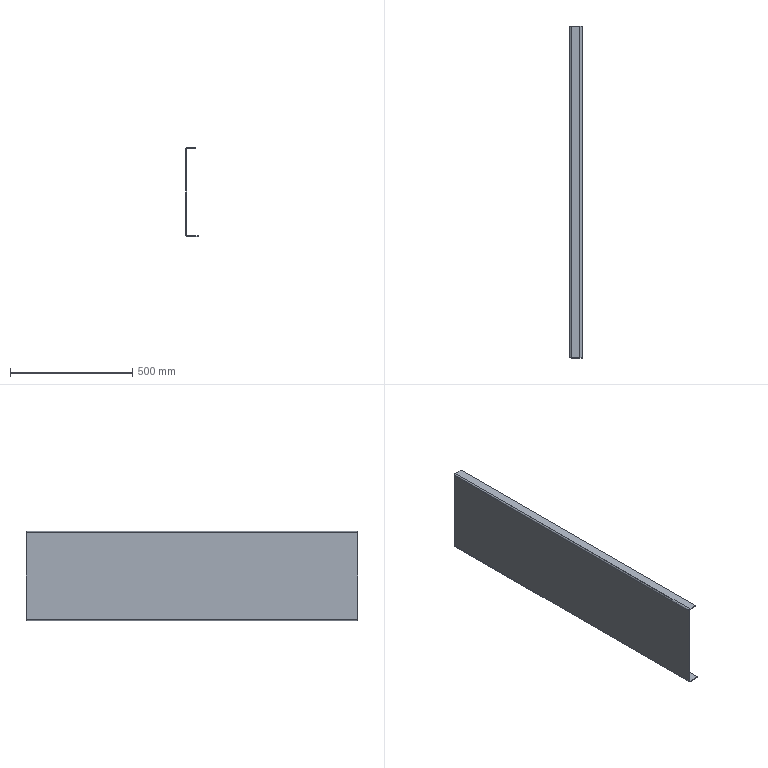Part | STEP file | VD-SYL0380DJ1006_1_1-3_VD-SYL03 | 1 solid | 14 faces | box 50 x 1360 x 365 mm | volume 1816160 mm3 | plane 10 | cylinder 4 | commonest cylinder face diameters 6 x2 12 x2
STEP:
#1=CARTESIAN_POINT('',(-17.,-680.,-3.));
#2=VERTEX_POINT('',#1);
#3=CARTESIAN_POINT('',(-14.,-680.,0.));
#4=VERTEX_POINT('',#3);
#5=CARTESIAN_POINT('',(-14.,-680.,-3.));
#6=DIRECTION('',(0.,1.,0.));
#7=DIRECTION('',(-1.,0.,0.));
#8=AXIS2_PLACEMENT_3D('',#5,#6,#7);
#9=CIRCLE('',#8,3.);
#10=EDGE_CURVE('',#2,#4,#9,.T.);
#11=ORIENTED_EDGE('',*,*,#10,.F.);
#12=CARTESIAN_POINT('',(-17.,680.,-3.));
#13=VERTEX_POINT('',#12);
#14=CARTESIAN_POINT('',(-17.,-680.,-3.));
#15=DIRECTION('',(0.,1.,0.));
#16=VECTOR('',#15,1000.);
#17=LINE('',#14,#16);
#18=EDGE_CURVE('',#2,#13,#17,.T.);
#19=ORIENTED_EDGE('',*,*,#18,.T.);
#20=CARTESIAN_POINT('',(-14.,680.,0.));
#21=VERTEX_POINT('',#20);
#22=CARTESIAN_POINT('',(-14.,680.,-3.));
#23=DIRECTION('',(0.,-1.,0.));
#24=DIRECTION('',(0.,0.,1.));
#25=AXIS2_PLACEMENT_3D('',#22,#23,#24);
#26=CIRCLE('',#25,3.);
#27=EDGE_CURVE('',#21,#13,#26,.T.);
#28=ORIENTED_EDGE('',*,*,#27,.F.);
#29=CARTESIAN_POINT('',(-14.,680.,0.));
#30=DIRECTION('',(0.,-1.,0.));
#31=VECTOR('',#30,1000.);
#32=LINE('',#29,#31);
#33=EDGE_CURVE('',#21,#4,#32,.T.);
#34=ORIENTED_EDGE('',*,*,#33,.T.);
#35=EDGE_LOOP('',(#11,#19,#28,#34));
#36=FACE_OUTER_BOUND('',#35,.T.);
#37=CARTESIAN_POINT('',(-14.,-680.,-3.));
#38=DIRECTION('',(0.,1.,0.));
#39=DIRECTION('',(0.,0.,1.));
#40=AXIS2_PLACEMENT_3D('',#37,#38,#39);
#41=CYLINDRICAL_SURFACE('',#40,3.);
#42=ADVANCED_FACE('',(#36),#41,.F.);
#43=CARTESIAN_POINT('',(20.,-680.,0.));
#44=VERTEX_POINT('',#43);
#45=CARTESIAN_POINT('',(20.,-680.,0.));
#46=DIRECTION('',(-1.,0.,0.));
#47=VECTOR('',#46,1000.);
#48=LINE('',#45,#47);
#49=EDGE_CURVE('',#44,#4,#48,.T.);
#50=ORIENTED_EDGE('',*,*,#49,.T.);
#51=ORIENTED_EDGE('',*,*,#33,.F.);
#52=CARTESIAN_POINT('',(20.,680.,0.));
#53=VERTEX_POINT('',#52);
#54=CARTESIAN_POINT('',(-14.,680.,0.));
#55=DIRECTION('',(1.,0.,0.));
#56=VECTOR('',#55,1000.);
#57=LINE('',#54,#56);
#58=EDGE_CURVE('',#21,#53,#57,.T.);
#59=ORIENTED_EDGE('',*,*,#58,.T.);
#60=CARTESIAN_POINT('',(20.,680.,0.));
#61=DIRECTION('',(0.,-1.,0.));
#62=VECTOR('',#61,1000.);
#63=LINE('',#60,#62);
#64=EDGE_CURVE('',#53,#44,#63,.T.);
#65=ORIENTED_EDGE('',*,*,#64,.T.);
#66=EDGE_LOOP('',(#50,#51,#59,#65));
#67=FACE_OUTER_BOUND('',#66,.T.);
#68=CARTESIAN_POINT('',(0.,0.,0.));
#69=DIRECTION('',(0.,0.,1.));
#70=DIRECTION('',(1.,0.,0.));
#71=AXIS2_PLACEMENT_3D('',#68,#69,#70);
#72=PLANE('',#71);
#73=ADVANCED_FACE('',(#67),#72,.F.);
#74=CARTESIAN_POINT('',(20.,-680.,3.));
#75=VERTEX_POINT('',#74);
#76=CARTESIAN_POINT('',(20.,-680.,3.));
#77=DIRECTION('',(0.,0.,-1.));
#78=VECTOR('',#77,1000.);
#79=LINE('',#76,#78);
#80=EDGE_CURVE('',#75,#44,#79,.T.);
#81=ORIENTED_EDGE('',*,*,#80,.T.);
#82=ORIENTED_EDGE('',*,*,#64,.F.);
#83=CARTESIAN_POINT('',(20.,680.,3.));
#84=VERTEX_POINT('',#83);
#85=CARTESIAN_POINT('',(20.,680.,3.));
#86=DIRECTION('',(0.,0.,-1.));
#87=VECTOR('',#86,1000.);
#88=LINE('',#85,#87);
#89=EDGE_CURVE('',#84,#53,#88,.T.);
#90=ORIENTED_EDGE('',*,*,#89,.F.);
#91=CARTESIAN_POINT('',(20.,680.,3.));
#92=DIRECTION('',(0.,-1.,0.));
#93=VECTOR('',#92,1000.);
#94=LINE('',#91,#93);
#95=EDGE_CURVE('',#84,#75,#94,.T.);
#96=ORIENTED_EDGE('',*,*,#95,.T.);
#97=EDGE_LOOP('',(#81,#82,#90,#96));
#98=FACE_OUTER_BOUND('',#97,.T.);
#99=CARTESIAN_POINT('',(20.,0.,1.5));
#100=DIRECTION('',(-1.,0.,0.));
#101=DIRECTION('',(0.,0.,1.));
#102=AXIS2_PLACEMENT_3D('',#99,#100,#101);
#103=PLANE('',#102);
#104=ADVANCED_FACE('',(#98),#103,.F.);
#105=CARTESIAN_POINT('',(-20.,680.,-3.));
#106=VERTEX_POINT('',#105);
#107=CARTESIAN_POINT('',(-20.,-680.,-3.));
#108=VERTEX_POINT('',#107);
#109=CARTESIAN_POINT('',(-20.,680.,-3.));
#110=DIRECTION('',(0.,-1.,0.));
#111=VECTOR('',#110,1000.);
#112=LINE('',#109,#111);
#113=EDGE_CURVE('',#106,#108,#112,.T.);
#114=ORIENTED_EDGE('',*,*,#113,.T.);
#115=CARTESIAN_POINT('',(-14.,-680.,3.));
#116=VERTEX_POINT('',#115);
#117=CARTESIAN_POINT('',(-14.,-680.,-3.));
#118=DIRECTION('',(0.,-1.,0.));
#119=DIRECTION('',(0.,0.,1.));
#120=AXIS2_PLACEMENT_3D('',#117,#118,#119);
#121=CIRCLE('',#120,6.);
#122=EDGE_CURVE('',#116,#108,#121,.T.);
#123=ORIENTED_EDGE('',*,*,#122,.F.);
#124=CARTESIAN_POINT('',(-14.,680.,3.));
#125=VERTEX_POINT('',#124);
#126=CARTESIAN_POINT('',(-14.,-680.,3.));
#127=DIRECTION('',(0.,1.,0.));
#128=VECTOR('',#127,1000.);
#129=LINE('',#126,#128);
#130=EDGE_CURVE('',#116,#125,#129,.T.);
#131=ORIENTED_EDGE('',*,*,#130,.T.);
#132=CARTESIAN_POINT('',(-14.,680.,-3.));
#133=DIRECTION('',(0.,1.,0.));
#134=DIRECTION('',(-1.,0.,0.));
#135=AXIS2_PLACEMENT_3D('',#132,#133,#134);
#136=CIRCLE('',#135,6.);
#137=EDGE_CURVE('',#106,#125,#136,.T.);
#138=ORIENTED_EDGE('',*,*,#137,.F.);
#139=EDGE_LOOP('',(#114,#123,#131,#138));
#140=FACE_OUTER_BOUND('',#139,.T.);
#141=CARTESIAN_POINT('',(-14.,-680.,-3.));
#142=DIRECTION('',(0.,1.,0.));
#143=DIRECTION('',(0.,0.,1.));
#144=AXIS2_PLACEMENT_3D('',#141,#142,#143);
#145=CYLINDRICAL_SURFACE('',#144,6.);
#146=ADVANCED_FACE('',(#140),#145,.T.);
#147=CARTESIAN_POINT('',(-20.,680.,-356.));
#148=VERTEX_POINT('',#147);
#149=CARTESIAN_POINT('',(-20.,680.,-3.));
#150=DIRECTION('',(0.,0.,-1.));
#151=VECTOR('',#150,1000.);
#152=LINE('',#149,#151);
#153=EDGE_CURVE('',#106,#148,#152,.T.);
#154=ORIENTED_EDGE('',*,*,#153,.T.);
#155=CARTESIAN_POINT('',(-20.,-680.,-356.));
#156=VERTEX_POINT('',#155);
#157=CARTESIAN_POINT('',(-20.,-680.,-356.));
#158=DIRECTION('',(0.,1.,0.));
#159=VECTOR('',#158,1000.);
#160=LINE('',#157,#159);
#161=EDGE_CURVE('',#156,#148,#160,.T.);
#162=ORIENTED_EDGE('',*,*,#161,.F.);
#163=CARTESIAN_POINT('',(-20.,-680.,-356.));
#164=DIRECTION('',(0.,0.,1.));
#165=VECTOR('',#164,1000.);
#166=LINE('',#163,#165);
#167=EDGE_CURVE('',#156,#108,#166,.T.);
#168=ORIENTED_EDGE('',*,*,#167,.T.);
#169=ORIENTED_EDGE('',*,*,#113,.F.);
#170=EDGE_LOOP('',(#154,#162,#168,#169));
#171=FACE_OUTER_BOUND('',#170,.T.);
#172=CARTESIAN_POINT('',(-20.,680.,3.));
#173=DIRECTION('',(-1.,0.,0.));
#174=DIRECTION('',(0.,0.,1.));
#175=AXIS2_PLACEMENT_3D('',#172,#173,#174);
#176=PLANE('',#175);
#177=ADVANCED_FACE('',(#171),#176,.T.);
#178=CARTESIAN_POINT('',(-14.,680.,-362.));
#179=VERTEX_POINT('',#178);
#180=CARTESIAN_POINT('',(-14.,-680.,-362.));
#181=VERTEX_POINT('',#180);
#182=CARTESIAN_POINT('',(-14.,680.,-362.));
#183=DIRECTION('',(0.,-1.,0.));
#184=VECTOR('',#183,1000.);
#185=LINE('',#182,#184);
#186=EDGE_CURVE('',#179,#181,#185,.T.);
#187=ORIENTED_EDGE('',*,*,#186,.T.);
#188=CARTESIAN_POINT('',(-14.,-680.,-356.));
#189=DIRECTION('',(0.,-1.,0.));
#190=DIRECTION('',(-1.,0.,0.));
#191=AXIS2_PLACEMENT_3D('',#188,#189,#190);
#192=CIRCLE('',#191,6.);
#193=EDGE_CURVE('',#156,#181,#192,.T.);
#194=ORIENTED_EDGE('',*,*,#193,.F.);
#195=ORIENTED_EDGE('',*,*,#161,.T.);
#196=CARTESIAN_POINT('',(-14.,680.,-356.));
#197=DIRECTION('',(0.,1.,0.));
#198=DIRECTION('',(0.,0.,-1.));
#199=AXIS2_PLACEMENT_3D('',#196,#197,#198);
#200=CIRCLE('',#199,6.);
#201=EDGE_CURVE('',#179,#148,#200,.T.);
#202=ORIENTED_EDGE('',*,*,#201,.F.);
#203=EDGE_LOOP('',(#187,#194,#195,#202));
#204=FACE_OUTER_BOUND('',#203,.T.);
#205=CARTESIAN_POINT('',(-14.,-680.,-356.));
#206=DIRECTION('',(0.,1.,0.));
#207=DIRECTION('',(0.,0.,1.));
#208=AXIS2_PLACEMENT_3D('',#205,#206,#207);
#209=CYLINDRICAL_SURFACE('',#208,6.);
#210=ADVANCED_FACE('',(#204),#209,.T.);
#211=CARTESIAN_POINT('',(30.,680.,-362.));
#212=VERTEX_POINT('',#211);
#213=CARTESIAN_POINT('',(-14.,680.,-362.));
#214=DIRECTION('',(1.,0.,0.));
#215=VECTOR('',#214,1000.);
#216=LINE('',#213,#215);
#217=EDGE_CURVE('',#179,#212,#216,.T.);
#218=ORIENTED_EDGE('',*,*,#217,.T.);
#219=CARTESIAN_POINT('',(30.,-680.,-362.));
#220=VERTEX_POINT('',#219);
#221=CARTESIAN_POINT('',(30.,680.,-362.));
#222=DIRECTION('',(0.,-1.,0.));
#223=VECTOR('',#222,1000.);
#224=LINE('',#221,#223);
#225=EDGE_CURVE('',#212,#220,#224,.T.);
#226=ORIENTED_EDGE('',*,*,#225,.T.);
#227=CARTESIAN_POINT('',(30.,-680.,-362.));
#228=DIRECTION('',(-1.,0.,0.));
#229=VECTOR('',#228,1000.);
#230=LINE('',#227,#229);
#231=EDGE_CURVE('',#220,#181,#230,.T.);
#232=ORIENTED_EDGE('',*,*,#231,.T.);
#233=ORIENTED_EDGE('',*,*,#186,.F.);
#234=EDGE_LOOP('',(#218,#226,#232,#233));
#235=FACE_OUTER_BOUND('',#234,.T.);
#236=CARTESIAN_POINT('',(-20.,680.,-362.));
#237=DIRECTION('',(0.,0.,-1.));
#238=DIRECTION('',(0.,-1.,0.));
#239=AXIS2_PLACEMENT_3D('',#236,#237,#238);
#240=PLANE('',#239);
#241=ADVANCED_FACE('',(#235),#240,.T.);
#242=ORIENTED_EDGE('',*,*,#225,.F.);
#243=CARTESIAN_POINT('',(30.,680.,-359.));
#244=VERTEX_POINT('',#243);
#245=CARTESIAN_POINT('',(30.,680.,-362.));
#246=DIRECTION('',(0.,0.,1.));
#247=VECTOR('',#246,1000.);
#248=LINE('',#245,#247);
#249=EDGE_CURVE('',#212,#244,#248,.T.);
#250=ORIENTED_EDGE('',*,*,#249,.T.);
#251=CARTESIAN_POINT('',(30.,-680.,-359.));
#252=VERTEX_POINT('',#251);
#253=CARTESIAN_POINT('',(30.,-680.,-359.));
#254=DIRECTION('',(0.,1.,0.));
#255=VECTOR('',#254,1000.);
#256=LINE('',#253,#255);
#257=EDGE_CURVE('',#252,#244,#256,.T.);
#258=ORIENTED_EDGE('',*,*,#257,.F.);
#259=CARTESIAN_POINT('',(30.,-680.,-359.));
#260=DIRECTION('',(0.,0.,-1.));
#261=VECTOR('',#260,1000.);
#262=LINE('',#259,#261);
#263=EDGE_CURVE('',#252,#220,#262,.T.);
#264=ORIENTED_EDGE('',*,*,#263,.T.);
#265=EDGE_LOOP('',(#242,#250,#258,#264));
#266=FACE_OUTER_BOUND('',#265,.T.);
#267=CARTESIAN_POINT('',(30.,0.,-360.5));
#268=DIRECTION('',(1.,0.,0.));
#269=DIRECTION('',(0.,1.,0.));
#270=AXIS2_PLACEMENT_3D('',#267,#268,#269);
#271=PLANE('',#270);
#272=ADVANCED_FACE('',(#266),#271,.T.);
#273=ORIENTED_EDGE('',*,*,#257,.T.);
#274=CARTESIAN_POINT('',(-14.,680.,-359.));
#275=VERTEX_POINT('',#274);
#276=CARTESIAN_POINT('',(30.,680.,-359.));
#277=DIRECTION('',(-1.,0.,0.));
#278=VECTOR('',#277,1000.);
#279=LINE('',#276,#278);
#280=EDGE_CURVE('',#244,#275,#279,.T.);
#281=ORIENTED_EDGE('',*,*,#280,.T.);
#282=CARTESIAN_POINT('',(-14.,-680.,-359.));
#283=VERTEX_POINT('',#282);
#284=CARTESIAN_POINT('',(-14.,-680.,-359.));
#285=DIRECTION('',(0.,1.,0.));
#286=VECTOR('',#285,1000.);
#287=LINE('',#284,#286);
#288=EDGE_CURVE('',#283,#275,#287,.T.);
#289=ORIENTED_EDGE('',*,*,#288,.F.);
#290=CARTESIAN_POINT('',(-14.,-680.,-359.));
#291=DIRECTION('',(1.,0.,0.));
#292=VECTOR('',#291,1000.);
#293=LINE('',#290,#292);
#294=EDGE_CURVE('',#283,#252,#293,.T.);
#295=ORIENTED_EDGE('',*,*,#294,.T.);
#296=EDGE_LOOP('',(#273,#281,#289,#295));
#297=FACE_OUTER_BOUND('',#296,.T.);
#298=CARTESIAN_POINT('',(-20.,680.,-359.));
#299=DIRECTION('',(0.,0.,-1.));
#300=DIRECTION('',(0.,-1.,0.));
#301=AXIS2_PLACEMENT_3D('',#298,#299,#300);
#302=PLANE('',#301);
#303=ADVANCED_FACE('',(#297),#302,.F.);
#304=CARTESIAN_POINT('',(-17.,-680.,-356.));
#305=VERTEX_POINT('',#304);
#306=CARTESIAN_POINT('',(-14.,-680.,-356.));
#307=DIRECTION('',(0.,1.,0.));
#308=DIRECTION('',(0.,0.,-1.));
#309=AXIS2_PLACEMENT_3D('',#306,#307,#308);
#310=CIRCLE('',#309,3.);
#311=EDGE_CURVE('',#283,#305,#310,.T.);
#312=ORIENTED_EDGE('',*,*,#311,.F.);
#313=ORIENTED_EDGE('',*,*,#288,.T.);
#314=CARTESIAN_POINT('',(-17.,680.,-356.));
#315=VERTEX_POINT('',#314);
#316=CARTESIAN_POINT('',(-14.,680.,-356.));
#317=DIRECTION('',(0.,-1.,0.));
#318=DIRECTION('',(-1.,0.,0.));
#319=AXIS2_PLACEMENT_3D('',#316,#317,#318);
#320=CIRCLE('',#319,3.);
#321=EDGE_CURVE('',#315,#275,#320,.T.);
#322=ORIENTED_EDGE('',*,*,#321,.F.);
#323=CARTESIAN_POINT('',(-17.,680.,-356.));
#324=DIRECTION('',(0.,-1.,0.));
#325=VECTOR('',#324,1000.);
#326=LINE('',#323,#325);
#327=EDGE_CURVE('',#315,#305,#326,.T.);
#328=ORIENTED_EDGE('',*,*,#327,.T.);
#329=EDGE_LOOP('',(#312,#313,#322,#328));
#330=FACE_OUTER_BOUND('',#329,.T.);
#331=CARTESIAN_POINT('',(-14.,-680.,-356.));
#332=DIRECTION('',(0.,1.,0.));
#333=DIRECTION('',(0.,0.,1.));
#334=AXIS2_PLACEMENT_3D('',#331,#332,#333);
#335=CYLINDRICAL_SURFACE('',#334,3.);
#336=ADVANCED_FACE('',(#330),#335,.F.);
#337=ORIENTED_EDGE('',*,*,#10,.T.);
#338=ORIENTED_EDGE('',*,*,#49,.F.);
#339=ORIENTED_EDGE('',*,*,#80,.F.);
#340=CARTESIAN_POINT('',(20.,-680.,3.));
#341=DIRECTION('',(-1.,0.,0.));
#342=VECTOR('',#341,1000.);
#343=LINE('',#340,#342);
#344=EDGE_CURVE('',#75,#116,#343,.T.);
#345=ORIENTED_EDGE('',*,*,#344,.T.);
#346=ORIENTED_EDGE('',*,*,#122,.T.);
#347=ORIENTED_EDGE('',*,*,#167,.F.);
#348=ORIENTED_EDGE('',*,*,#193,.T.);
#349=ORIENTED_EDGE('',*,*,#231,.F.);
#350=ORIENTED_EDGE('',*,*,#263,.F.);
#351=ORIENTED_EDGE('',*,*,#294,.F.);
#352=ORIENTED_EDGE('',*,*,#311,.T.);
#353=CARTESIAN_POINT('',(-17.,-680.,-3.));
#354=DIRECTION('',(0.,0.,-1.));
#355=VECTOR('',#354,1000.);
#356=LINE('',#353,#355);
#357=EDGE_CURVE('',#2,#305,#356,.T.);
#358=ORIENTED_EDGE('',*,*,#357,.F.);
#359=EDGE_LOOP('',(#337,#338,#339,#345,#346,#347,#348,#349,#350,#351,#352,#358));
#360=FACE_OUTER_BOUND('',#359,.T.);
#361=CARTESIAN_POINT('',(-18.5,-680.,-182.5));
#362=DIRECTION('',(0.,-1.,0.));
#363=DIRECTION('',(0.,0.,-1.));
#364=AXIS2_PLACEMENT_3D('',#361,#362,#363);
#365=PLANE('',#364);
#366=ADVANCED_FACE('',(#360),#365,.T.);
#367=ORIENTED_EDGE('',*,*,#327,.F.);
#368=CARTESIAN_POINT('',(-17.,680.,-356.));
#369=DIRECTION('',(0.,0.,1.));
#370=VECTOR('',#369,1000.);
#371=LINE('',#368,#370);
#372=EDGE_CURVE('',#315,#13,#371,.T.);
#373=ORIENTED_EDGE('',*,*,#372,.T.);
#374=ORIENTED_EDGE('',*,*,#18,.F.);
#375=ORIENTED_EDGE('',*,*,#357,.T.);
#376=EDGE_LOOP('',(#367,#373,#374,#375));
#377=FACE_OUTER_BOUND('',#376,.T.);
#378=CARTESIAN_POINT('',(-17.,680.,3.));
#379=DIRECTION('',(-1.,0.,0.));
#380=DIRECTION('',(0.,0.,1.));
#381=AXIS2_PLACEMENT_3D('',#378,#379,#380);
#382=PLANE('',#381);
#383=ADVANCED_FACE('',(#377),#382,.F.);
#384=ORIENTED_EDGE('',*,*,#321,.T.);
#385=ORIENTED_EDGE('',*,*,#280,.F.);
#386=ORIENTED_EDGE('',*,*,#249,.F.);
#387=ORIENTED_EDGE('',*,*,#217,.F.);
#388=ORIENTED_EDGE('',*,*,#201,.T.);
#389=ORIENTED_EDGE('',*,*,#153,.F.);
#390=ORIENTED_EDGE('',*,*,#137,.T.);
#391=CARTESIAN_POINT('',(-14.,680.,3.));
#392=DIRECTION('',(1.,0.,0.));
#393=VECTOR('',#392,1000.);
#394=LINE('',#391,#393);
#395=EDGE_CURVE('',#125,#84,#394,.T.);
#396=ORIENTED_EDGE('',*,*,#395,.T.);
#397=ORIENTED_EDGE('',*,*,#89,.T.);
#398=ORIENTED_EDGE('',*,*,#58,.F.);
#399=ORIENTED_EDGE('',*,*,#27,.T.);
#400=ORIENTED_EDGE('',*,*,#372,.F.);
#401=EDGE_LOOP('',(#384,#385,#386,#387,#388,#389,#390,#396,#397,#398,#399,#400));
#402=FACE_OUTER_BOUND('',#401,.T.);
#403=CARTESIAN_POINT('',(-18.5,680.,-182.5));
#404=DIRECTION('',(0.,1.,0.));
#405=DIRECTION('',(1.,0.,0.));
#406=AXIS2_PLACEMENT_3D('',#403,#404,#405);
#407=PLANE('',#406);
#408=ADVANCED_FACE('',(#402),#407,.T.);
#409=ORIENTED_EDGE('',*,*,#130,.F.);
#410=ORIENTED_EDGE('',*,*,#344,.F.);
#411=ORIENTED_EDGE('',*,*,#95,.F.);
#412=ORIENTED_EDGE('',*,*,#395,.F.);
#413=EDGE_LOOP('',(#409,#410,#411,#412));
#414=FACE_OUTER_BOUND('',#413,.T.);
#415=CARTESIAN_POINT('',(0.,0.,3.));
#416=DIRECTION('',(0.,0.,1.));
#417=DIRECTION('',(1.,0.,0.));
#418=AXIS2_PLACEMENT_3D('',#415,#416,#417);
#419=PLANE('',#418);
#420=ADVANCED_FACE('',(#414),#419,.T.);
#421=CLOSED_SHELL('',(#42,#73,#104,#146,#177,#210,#241,#272,#303,#336,#366,#383,#408,#420));
#422=MANIFOLD_SOLID_BREP('',#421);
#423=CARTESIAN_POINT('',(0.,0.,0.));
#424=DIRECTION('',(0.,0.,1.));
#425=DIRECTION('',(1.,0.,0.));
#426=AXIS2_PLACEMENT_3D('',#423,#424,#425);
#427=(LENGTH_UNIT()NAMED_UNIT(*)SI_UNIT(.MILLI.,.METRE.));
#428=UNCERTAINTY_MEASURE_WITH_UNIT(LENGTH_MEASURE(0.00001),#427,'','');
#429=(NAMED_UNIT(*)PLANE_ANGLE_UNIT()SI_UNIT($,.RADIAN.));
#430=(NAMED_UNIT(*)SI_UNIT($,.STERADIAN.)SOLID_ANGLE_UNIT());
#431=(GEOMETRIC_REPRESENTATION_CONTEXT(3)GLOBAL_UNCERTAINTY_ASSIGNED_CONTEXT((#428))GLOBAL_UNIT_ASSIGNED_CONTEXT((#427,#429,#430))REPRESENTATION_CONTEXT('',''));
#432=ADVANCED_BREP_SHAPE_REPRESENTATION('',(#422,#426),#431);